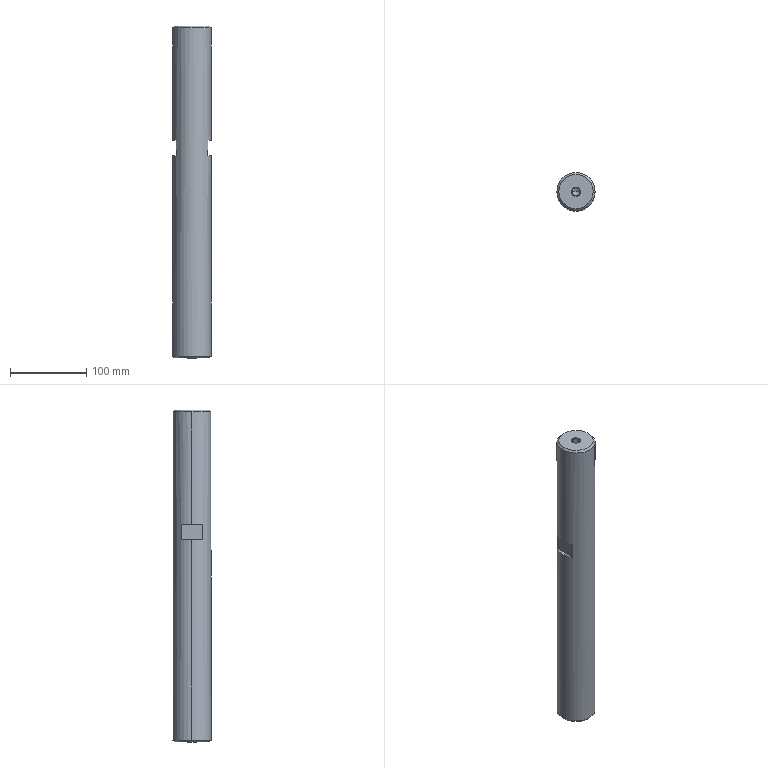Part | STEP file | RAD36-D50-L435-SC150-M12-N12-Yiheda | 1 solid | 26 faces | box 50 x 50 x 435 mm | volume 845554 mm3 | cone 12 | plane 8 | cylinder 6 | commonest cylinder face diameters 10.106 x4 50 x2
STEP:
#1=CARTESIAN_POINT('',(-25.,0.,-2.5));
#2=VERTEX_POINT('',#1);
#3=CARTESIAN_POINT('',(25.,0.,-2.5));
#4=VERTEX_POINT('',#3);
#5=CARTESIAN_POINT('',(0.,0.,-2.5));
#6=DIRECTION('',(0.,0.,-1.));
#7=DIRECTION('',(-1.,0.,0.));
#8=AXIS2_PLACEMENT_3D('',#5,#6,#7);
#9=CIRCLE('',#8,25.);
#10=EDGE_CURVE('',#2,#4,#9,.T.);
#11=ORIENTED_EDGE('',*,*,#10,.T.);
#12=CARTESIAN_POINT('',(25.,0.,-150.));
#13=VERTEX_POINT('',#12);
#14=CARTESIAN_POINT('',(25.,0.,-600.));
#15=DIRECTION('',(0.,0.,-1.));
#16=VECTOR('',#15,1000.);
#17=LINE('',#14,#16);
#18=EDGE_CURVE('',#4,#13,#17,.T.);
#19=ORIENTED_EDGE('',*,*,#18,.T.);
#20=CARTESIAN_POINT('',(20.5,14.309,-150.));
#21=VERTEX_POINT('',#20);
#22=CARTESIAN_POINT('',(0.,0.,-150.));
#23=DIRECTION('',(0.,0.,1.));
#24=DIRECTION('',(-1.,0.,0.));
#25=AXIS2_PLACEMENT_3D('',#22,#23,#24);
#26=CIRCLE('',#25,25.);
#27=EDGE_CURVE('',#13,#21,#26,.T.);
#28=ORIENTED_EDGE('',*,*,#27,.T.);
#29=CARTESIAN_POINT('',(20.5,14.309,-170.));
#30=VERTEX_POINT('',#29);
#31=CARTESIAN_POINT('',(20.5,14.309,-600.));
#32=DIRECTION('',(0.,0.,-1.));
#33=VECTOR('',#32,1000.);
#34=LINE('',#31,#33);
#35=EDGE_CURVE('',#21,#30,#34,.T.);
#36=ORIENTED_EDGE('',*,*,#35,.T.);
#37=CARTESIAN_POINT('',(25.,0.,-170.));
#38=VERTEX_POINT('',#37);
#39=CARTESIAN_POINT('',(0.,0.,-170.));
#40=DIRECTION('',(0.,0.,-1.));
#41=DIRECTION('',(-1.,0.,0.));
#42=AXIS2_PLACEMENT_3D('',#39,#40,#41);
#43=CIRCLE('',#42,25.);
#44=EDGE_CURVE('',#30,#38,#43,.T.);
#45=ORIENTED_EDGE('',*,*,#44,.T.);
#46=CARTESIAN_POINT('',(25.,0.,-432.5));
#47=VERTEX_POINT('',#46);
#48=CARTESIAN_POINT('',(25.,0.,-600.));
#49=DIRECTION('',(0.,0.,-1.));
#50=VECTOR('',#49,1000.);
#51=LINE('',#48,#50);
#52=EDGE_CURVE('',#38,#47,#51,.T.);
#53=ORIENTED_EDGE('',*,*,#52,.T.);
#54=CARTESIAN_POINT('',(0.,25.,-432.5));
#55=VERTEX_POINT('',#54);
#56=CARTESIAN_POINT('',(0.,0.,-432.5));
#57=DIRECTION('',(0.,0.,1.));
#58=DIRECTION('',(-1.,0.,0.));
#59=AXIS2_PLACEMENT_3D('',#56,#57,#58);
#60=CIRCLE('',#59,25.);
#61=EDGE_CURVE('',#47,#55,#60,.T.);
#62=ORIENTED_EDGE('',*,*,#61,.T.);
#63=CARTESIAN_POINT('',(-25.,0.,-432.5));
#64=VERTEX_POINT('',#63);
#65=CARTESIAN_POINT('',(0.,0.,-432.5));
#66=DIRECTION('',(0.,0.,1.));
#67=DIRECTION('',(-1.,0.,0.));
#68=AXIS2_PLACEMENT_3D('',#65,#66,#67);
#69=CIRCLE('',#68,25.);
#70=EDGE_CURVE('',#55,#64,#69,.T.);
#71=ORIENTED_EDGE('',*,*,#70,.T.);
#72=CARTESIAN_POINT('',(-25.,0.,-170.));
#73=VERTEX_POINT('',#72);
#74=CARTESIAN_POINT('',(-25.,0.,-600.));
#75=DIRECTION('',(0.,0.,-1.));
#76=VECTOR('',#75,1000.);
#77=LINE('',#74,#76);
#78=EDGE_CURVE('',#73,#64,#77,.T.);
#79=ORIENTED_EDGE('',*,*,#78,.F.);
#80=CARTESIAN_POINT('',(-20.5,14.309,-170.));
#81=VERTEX_POINT('',#80);
#82=CARTESIAN_POINT('',(0.,0.,-170.));
#83=DIRECTION('',(0.,0.,-1.));
#84=DIRECTION('',(-1.,0.,0.));
#85=AXIS2_PLACEMENT_3D('',#82,#83,#84);
#86=CIRCLE('',#85,25.);
#87=EDGE_CURVE('',#73,#81,#86,.T.);
#88=ORIENTED_EDGE('',*,*,#87,.T.);
#89=CARTESIAN_POINT('',(-20.5,14.309,-150.));
#90=VERTEX_POINT('',#89);
#91=CARTESIAN_POINT('',(-20.5,14.309,-600.));
#92=DIRECTION('',(0.,0.,1.));
#93=VECTOR('',#92,1000.);
#94=LINE('',#91,#93);
#95=EDGE_CURVE('',#81,#90,#94,.T.);
#96=ORIENTED_EDGE('',*,*,#95,.T.);
#97=CARTESIAN_POINT('',(-25.,0.,-150.));
#98=VERTEX_POINT('',#97);
#99=CARTESIAN_POINT('',(0.,0.,-150.));
#100=DIRECTION('',(0.,0.,1.));
#101=DIRECTION('',(-1.,0.,0.));
#102=AXIS2_PLACEMENT_3D('',#99,#100,#101);
#103=CIRCLE('',#102,25.);
#104=EDGE_CURVE('',#90,#98,#103,.T.);
#105=ORIENTED_EDGE('',*,*,#104,.T.);
#106=CARTESIAN_POINT('',(-25.,0.,-600.));
#107=DIRECTION('',(0.,0.,-1.));
#108=VECTOR('',#107,1000.);
#109=LINE('',#106,#108);
#110=EDGE_CURVE('',#2,#98,#109,.T.);
#111=ORIENTED_EDGE('',*,*,#110,.F.);
#112=EDGE_LOOP('',(#11,#19,#28,#36,#45,#53,#62,#71,#79,#88,#96,#105,#111));
#113=FACE_OUTER_BOUND('',#112,.T.);
#114=CARTESIAN_POINT('',(0.,0.,-600.));
#115=DIRECTION('',(0.,0.,-1.));
#116=DIRECTION('',(-1.,0.,0.));
#117=AXIS2_PLACEMENT_3D('',#114,#115,#116);
#118=CYLINDRICAL_SURFACE('',#117,25.);
#119=ADVANCED_FACE('',(#113),#118,.T.);
#120=CARTESIAN_POINT('',(-22.5,0.,0.));
#121=VERTEX_POINT('',#120);
#122=CARTESIAN_POINT('',(22.5,0.,0.));
#123=VERTEX_POINT('',#122);
#124=CARTESIAN_POINT('',(0.,0.,0.));
#125=DIRECTION('',(0.,0.,-1.));
#126=DIRECTION('',(-1.,0.,0.));
#127=AXIS2_PLACEMENT_3D('',#124,#125,#126);
#128=CIRCLE('',#127,22.5);
#129=EDGE_CURVE('',#121,#123,#128,.T.);
#130=ORIENTED_EDGE('',*,*,#129,.T.);
#131=CARTESIAN_POINT('',(25.,0.,-2.5));
#132=DIRECTION('',(0.7071,0.,-0.7071));
#133=VECTOR('',#132,1000.);
#134=LINE('',#131,#133);
#135=EDGE_CURVE('',#123,#4,#134,.T.);
#136=ORIENTED_EDGE('',*,*,#135,.T.);
#137=ORIENTED_EDGE('',*,*,#10,.F.);
#138=CARTESIAN_POINT('',(-25.,0.,-2.5));
#139=DIRECTION('',(-0.7071,0.,-0.7071));
#140=VECTOR('',#139,1000.);
#141=LINE('',#138,#140);
#142=EDGE_CURVE('',#121,#2,#141,.T.);
#143=ORIENTED_EDGE('',*,*,#142,.F.);
#144=EDGE_LOOP('',(#130,#136,#137,#143));
#145=FACE_OUTER_BOUND('',#144,.T.);
#146=CARTESIAN_POINT('',(0.,0.,-2.5));
#147=DIRECTION('',(0.,0.,-1.));
#148=DIRECTION('',(-1.,0.,0.));
#149=AXIS2_PLACEMENT_3D('',#146,#147,#148);
#150=CONICAL_SURFACE('',#149,25.,0.7854);
#151=ADVANCED_FACE('',(#145),#150,.T.);
#152=CARTESIAN_POINT('',(0.,-22.5,-435.));
#153=VERTEX_POINT('',#152);
#154=CARTESIAN_POINT('',(0.,22.5,-435.));
#155=VERTEX_POINT('',#154);
#156=CARTESIAN_POINT('',(0.,0.,-435.));
#157=DIRECTION('',(0.,0.,1.));
#158=DIRECTION('',(0.,-1.,0.));
#159=AXIS2_PLACEMENT_3D('',#156,#157,#158);
#160=CIRCLE('',#159,22.5);
#161=EDGE_CURVE('',#153,#155,#160,.T.);
#162=ORIENTED_EDGE('',*,*,#161,.T.);
#163=CARTESIAN_POINT('',(0.,25.,-432.5));
#164=DIRECTION('',(0.,0.7071,0.7071));
#165=VECTOR('',#164,1000.);
#166=LINE('',#163,#165);
#167=EDGE_CURVE('',#155,#55,#166,.T.);
#168=ORIENTED_EDGE('',*,*,#167,.T.);
#169=ORIENTED_EDGE('',*,*,#61,.F.);
#170=CARTESIAN_POINT('',(0.,-25.,-432.5));
#171=VERTEX_POINT('',#170);
#172=CARTESIAN_POINT('',(0.,0.,-432.5));
#173=DIRECTION('',(0.,0.,1.));
#174=DIRECTION('',(-1.,0.,0.));
#175=AXIS2_PLACEMENT_3D('',#172,#173,#174);
#176=CIRCLE('',#175,25.);
#177=EDGE_CURVE('',#171,#47,#176,.T.);
#178=ORIENTED_EDGE('',*,*,#177,.F.);
#179=CARTESIAN_POINT('',(0.,-25.,-432.5));
#180=DIRECTION('',(0.,-0.7071,0.7071));
#181=VECTOR('',#180,1000.);
#182=LINE('',#179,#181);
#183=EDGE_CURVE('',#153,#171,#182,.T.);
#184=ORIENTED_EDGE('',*,*,#183,.F.);
#185=EDGE_LOOP('',(#162,#168,#169,#178,#184));
#186=FACE_OUTER_BOUND('',#185,.T.);
#187=CARTESIAN_POINT('',(0.,0.,-432.5));
#188=DIRECTION('',(0.,0.,1.));
#189=DIRECTION('',(0.,-1.,0.));
#190=AXIS2_PLACEMENT_3D('',#187,#188,#189);
#191=CONICAL_SURFACE('',#190,25.,0.7854);
#192=ADVANCED_FACE('',(#186),#191,.T.);
#193=CARTESIAN_POINT('',(0.,5.053,-0.947));
#194=VERTEX_POINT('',#193);
#195=CARTESIAN_POINT('',(0.,-5.053,-0.947));
#196=VERTEX_POINT('',#195);
#197=CARTESIAN_POINT('',(0.,0.,-0.947));
#198=DIRECTION('',(0.,0.,1.));
#199=DIRECTION('',(0.,-1.,0.));
#200=AXIS2_PLACEMENT_3D('',#197,#198,#199);
#201=CIRCLE('',#200,5.053);
#202=EDGE_CURVE('',#194,#196,#201,.T.);
#203=ORIENTED_EDGE('',*,*,#202,.F.);
#204=CARTESIAN_POINT('',(0.,6.,0.));
#205=VERTEX_POINT('',#204);
#206=CARTESIAN_POINT('',(0.,6.,0.));
#207=DIRECTION('',(0.,0.7071,0.7071));
#208=VECTOR('',#207,1000.);
#209=LINE('',#206,#208);
#210=EDGE_CURVE('',#194,#205,#209,.T.);
#211=ORIENTED_EDGE('',*,*,#210,.T.);
#212=CARTESIAN_POINT('',(0.,-6.,0.));
#213=VERTEX_POINT('',#212);
#214=CARTESIAN_POINT('',(0.,0.,0.));
#215=DIRECTION('',(0.,0.,1.));
#216=DIRECTION('',(0.,-1.,0.));
#217=AXIS2_PLACEMENT_3D('',#214,#215,#216);
#218=CIRCLE('',#217,6.);
#219=EDGE_CURVE('',#205,#213,#218,.T.);
#220=ORIENTED_EDGE('',*,*,#219,.T.);
#221=CARTESIAN_POINT('',(0.,-6.,0.));
#222=DIRECTION('',(0.,-0.7071,0.7071));
#223=VECTOR('',#222,1000.);
#224=LINE('',#221,#223);
#225=EDGE_CURVE('',#196,#213,#224,.T.);
#226=ORIENTED_EDGE('',*,*,#225,.F.);
#227=EDGE_LOOP('',(#203,#211,#220,#226));
#228=FACE_OUTER_BOUND('',#227,.T.);
#229=CARTESIAN_POINT('',(0.,0.,0.));
#230=DIRECTION('',(0.,0.,1.));
#231=DIRECTION('',(0.,-1.,0.));
#232=AXIS2_PLACEMENT_3D('',#229,#230,#231);
#233=CONICAL_SURFACE('',#232,6.,0.7854);
#234=ADVANCED_FACE('',(#228),#233,.F.);
#235=CARTESIAN_POINT('',(5.053,0.,-434.053));
#236=VERTEX_POINT('',#235);
#237=CARTESIAN_POINT('',(0.,-5.053,-434.053));
#238=VERTEX_POINT('',#237);
#239=CARTESIAN_POINT('',(0.,0.,-434.053));
#240=DIRECTION('',(0.,0.,-1.));
#241=DIRECTION('',(0.,1.,0.));
#242=AXIS2_PLACEMENT_3D('',#239,#240,#241);
#243=CIRCLE('',#242,5.053);
#244=EDGE_CURVE('',#236,#238,#243,.T.);
#245=ORIENTED_EDGE('',*,*,#244,.F.);
#246=CARTESIAN_POINT('',(6.,0.,-435.));
#247=VERTEX_POINT('',#246);
#248=CARTESIAN_POINT('',(6.,0.,-435.));
#249=DIRECTION('',(0.7071,0.,-0.7071));
#250=VECTOR('',#249,1000.);
#251=LINE('',#248,#250);
#252=EDGE_CURVE('',#236,#247,#251,.T.);
#253=ORIENTED_EDGE('',*,*,#252,.T.);
#254=CARTESIAN_POINT('',(-6.,0.,-435.));
#255=VERTEX_POINT('',#254);
#256=CARTESIAN_POINT('',(0.,0.,-435.));
#257=DIRECTION('',(0.,0.,-1.));
#258=DIRECTION('',(-1.,0.,0.));
#259=AXIS2_PLACEMENT_3D('',#256,#257,#258);
#260=CIRCLE('',#259,6.);
#261=EDGE_CURVE('',#247,#255,#260,.T.);
#262=ORIENTED_EDGE('',*,*,#261,.T.);
#263=CARTESIAN_POINT('',(-5.053,0.,-434.053));
#264=VERTEX_POINT('',#263);
#265=CARTESIAN_POINT('',(-6.,0.,-435.));
#266=DIRECTION('',(-0.7071,0.,-0.7071));
#267=VECTOR('',#266,1000.);
#268=LINE('',#265,#267);
#269=EDGE_CURVE('',#264,#255,#268,.T.);
#270=ORIENTED_EDGE('',*,*,#269,.F.);
#271=CARTESIAN_POINT('',(0.,0.,-434.053));
#272=DIRECTION('',(0.,0.,-1.));
#273=DIRECTION('',(0.,1.,0.));
#274=AXIS2_PLACEMENT_3D('',#271,#272,#273);
#275=CIRCLE('',#274,5.053);
#276=EDGE_CURVE('',#238,#264,#275,.T.);
#277=ORIENTED_EDGE('',*,*,#276,.F.);
#278=EDGE_LOOP('',(#245,#253,#262,#270,#277));
#279=FACE_OUTER_BOUND('',#278,.T.);
#280=CARTESIAN_POINT('',(0.,0.,-435.));
#281=DIRECTION('',(0.,0.,-1.));
#282=DIRECTION('',(-1.,0.,0.));
#283=AXIS2_PLACEMENT_3D('',#280,#281,#282);
#284=CONICAL_SURFACE('',#283,6.,0.7854);
#285=ADVANCED_FACE('',(#279),#284,.F.);
#286=ORIENTED_EDGE('',*,*,#202,.T.);
#287=CARTESIAN_POINT('',(0.,-5.053,-24.5));
#288=VERTEX_POINT('',#287);
#289=CARTESIAN_POINT('',(0.,-5.053,-27.417));
#290=DIRECTION('',(0.,0.,-1.));
#291=VECTOR('',#290,1000.);
#292=LINE('',#289,#291);
#293=EDGE_CURVE('',#196,#288,#292,.T.);
#294=ORIENTED_EDGE('',*,*,#293,.T.);
#295=CARTESIAN_POINT('',(-5.053,0.,-24.5));
#296=VERTEX_POINT('',#295);
#297=CARTESIAN_POINT('',(0.,0.,-24.5));
#298=DIRECTION('',(0.,0.,1.));
#299=DIRECTION('',(0.,1.,0.));
#300=AXIS2_PLACEMENT_3D('',#297,#298,#299);
#301=CIRCLE('',#300,5.053);
#302=EDGE_CURVE('',#296,#288,#301,.T.);
#303=ORIENTED_EDGE('',*,*,#302,.F.);
#304=CARTESIAN_POINT('',(0.,5.053,-24.5));
#305=VERTEX_POINT('',#304);
#306=CARTESIAN_POINT('',(0.,0.,-24.5));
#307=DIRECTION('',(0.,0.,1.));
#308=DIRECTION('',(0.,1.,0.));
#309=AXIS2_PLACEMENT_3D('',#306,#307,#308);
#310=CIRCLE('',#309,5.053);
#311=EDGE_CURVE('',#305,#296,#310,.T.);
#312=ORIENTED_EDGE('',*,*,#311,.F.);
#313=CARTESIAN_POINT('',(0.,5.053,-27.417));
#314=DIRECTION('',(0.,0.,-1.));
#315=VECTOR('',#314,1000.);
#316=LINE('',#313,#315);
#317=EDGE_CURVE('',#194,#305,#316,.T.);
#318=ORIENTED_EDGE('',*,*,#317,.F.);
#319=EDGE_LOOP('',(#286,#294,#303,#312,#318));
#320=FACE_OUTER_BOUND('',#319,.T.);
#321=CARTESIAN_POINT('',(0.,0.,-27.417));
#322=DIRECTION('',(0.,0.,-1.));
#323=DIRECTION('',(0.,1.,0.));
#324=AXIS2_PLACEMENT_3D('',#321,#322,#323);
#325=CYLINDRICAL_SURFACE('',#324,5.053);
#326=ADVANCED_FACE('',(#320),#325,.F.);
#327=CARTESIAN_POINT('',(0.,-5.053,-410.5));
#328=VERTEX_POINT('',#327);
#329=CARTESIAN_POINT('',(-5.053,0.,-410.5));
#330=VERTEX_POINT('',#329);
#331=CARTESIAN_POINT('',(0.,0.,-410.5));
#332=DIRECTION('',(0.,0.,-1.));
#333=DIRECTION('',(0.,1.,0.));
#334=AXIS2_PLACEMENT_3D('',#331,#332,#333);
#335=CIRCLE('',#334,5.053);
#336=EDGE_CURVE('',#328,#330,#335,.T.);
#337=ORIENTED_EDGE('',*,*,#336,.F.);
#338=CARTESIAN_POINT('',(0.,-5.053,-435.));
#339=DIRECTION('',(0.,0.,-1.));
#340=VECTOR('',#339,1000.);
#341=LINE('',#338,#340);
#342=EDGE_CURVE('',#328,#238,#341,.T.);
#343=ORIENTED_EDGE('',*,*,#342,.T.);
#344=ORIENTED_EDGE('',*,*,#276,.T.);
#345=CARTESIAN_POINT('',(0.,5.053,-434.053));
#346=VERTEX_POINT('',#345);
#347=CARTESIAN_POINT('',(0.,0.,-434.053));
#348=DIRECTION('',(0.,0.,-1.));
#349=DIRECTION('',(0.,1.,0.));
#350=AXIS2_PLACEMENT_3D('',#347,#348,#349);
#351=CIRCLE('',#350,5.053);
#352=EDGE_CURVE('',#264,#346,#351,.T.);
#353=ORIENTED_EDGE('',*,*,#352,.T.);
#354=CARTESIAN_POINT('',(0.,5.053,-410.5));
#355=VERTEX_POINT('',#354);
#356=CARTESIAN_POINT('',(0.,5.053,-435.));
#357=DIRECTION('',(0.,0.,-1.));
#358=VECTOR('',#357,1000.);
#359=LINE('',#356,#358);
#360=EDGE_CURVE('',#355,#346,#359,.T.);
#361=ORIENTED_EDGE('',*,*,#360,.F.);
#362=CARTESIAN_POINT('',(0.,0.,-410.5));
#363=DIRECTION('',(0.,0.,-1.));
#364=DIRECTION('',(0.,1.,0.));
#365=AXIS2_PLACEMENT_3D('',#362,#363,#364);
#366=CIRCLE('',#365,5.053);
#367=EDGE_CURVE('',#330,#355,#366,.T.);
#368=ORIENTED_EDGE('',*,*,#367,.F.);
#369=EDGE_LOOP('',(#337,#343,#344,#353,#361,#368));
#370=FACE_OUTER_BOUND('',#369,.T.);
#371=CARTESIAN_POINT('',(0.,0.,-435.));
#372=DIRECTION('',(0.,0.,-1.));
#373=DIRECTION('',(0.,1.,0.));
#374=AXIS2_PLACEMENT_3D('',#371,#372,#373);
#375=CYLINDRICAL_SURFACE('',#374,5.053);
#376=ADVANCED_FACE('',(#370),#375,.F.);
#377=CARTESIAN_POINT('',(0.,0.,-27.417));
#378=VERTEX_POINT('',#377);
#379=CARTESIAN_POINT('',(5.053,0.,-24.5));
#380=VERTEX_POINT('',#379);
#381=CARTESIAN_POINT('',(5.053,0.,-24.5));
#382=DIRECTION('',(0.866,0.,0.5));
#383=VECTOR('',#382,1000.);
#384=LINE('',#381,#383);
#385=EDGE_CURVE('',#378,#380,#384,.T.);
#386=ORIENTED_EDGE('',*,*,#385,.F.);
#387=CARTESIAN_POINT('',(-5.053,0.,-24.5));
#388=DIRECTION('',(-0.866,0.,0.5));
#389=VECTOR('',#388,1000.);
#390=LINE('',#387,#389);
#391=EDGE_CURVE('',#378,#296,#390,.T.);
#392=ORIENTED_EDGE('',*,*,#391,.T.);
#393=ORIENTED_EDGE('',*,*,#302,.T.);
#394=CARTESIAN_POINT('',(0.,0.,-24.5));
#395=DIRECTION('',(0.,0.,1.));
#396=DIRECTION('',(0.,1.,0.));
#397=AXIS2_PLACEMENT_3D('',#394,#395,#396);
#398=CIRCLE('',#397,5.053);
#399=EDGE_CURVE('',#288,#380,#398,.T.);
#400=ORIENTED_EDGE('',*,*,#399,.T.);
#401=EDGE_LOOP('',(#386,#392,#393,#400));
#402=FACE_OUTER_BOUND('',#401,.T.);
#403=CARTESIAN_POINT('',(0.,0.,-24.5));
#404=DIRECTION('',(0.,0.,1.));
#405=DIRECTION('',(1.,0.,0.));
#406=AXIS2_PLACEMENT_3D('',#403,#404,#405);
#407=CONICAL_SURFACE('',#406,5.053,1.047);
#408=ADVANCED_FACE('',(#402),#407,.F.);
#409=CARTESIAN_POINT('',(0.,0.,-407.583));
#410=VERTEX_POINT('',#409);
#411=CARTESIAN_POINT('',(-5.053,0.,-410.5));
#412=DIRECTION('',(-0.866,0.,-0.5));
#413=VECTOR('',#412,1000.);
#414=LINE('',#411,#413);
#415=EDGE_CURVE('',#410,#330,#414,.T.);
#416=ORIENTED_EDGE('',*,*,#415,.F.);
#417=CARTESIAN_POINT('',(5.053,0.,-410.5));
#418=VERTEX_POINT('',#417);
#419=CARTESIAN_POINT('',(5.053,0.,-410.5));
#420=DIRECTION('',(0.866,0.,-0.5));
#421=VECTOR('',#420,1000.);
#422=LINE('',#419,#421);
#423=EDGE_CURVE('',#410,#418,#422,.T.);
#424=ORIENTED_EDGE('',*,*,#423,.T.);
#425=CARTESIAN_POINT('',(0.,0.,-410.5));
#426=DIRECTION('',(0.,0.,-1.));
#427=DIRECTION('',(0.,1.,0.));
#428=AXIS2_PLACEMENT_3D('',#425,#426,#427);
#429=CIRCLE('',#428,5.053);
#430=EDGE_CURVE('',#418,#328,#429,.T.);
#431=ORIENTED_EDGE('',*,*,#430,.T.);
#432=ORIENTED_EDGE('',*,*,#336,.T.);
#433=EDGE_LOOP('',(#416,#424,#431,#432));
#434=FACE_OUTER_BOUND('',#433,.T.);
#435=CARTESIAN_POINT('',(0.,0.,-410.5));
#436=DIRECTION('',(0.,0.,-1.));
#437=DIRECTION('',(-1.,0.,0.));
#438=AXIS2_PLACEMENT_3D('',#435,#436,#437);
#439=CONICAL_SURFACE('',#438,5.053,1.047);
#440=ADVANCED_FACE('',(#434),#439,.F.);
#441=ORIENTED_EDGE('',*,*,#18,.F.);
#442=CARTESIAN_POINT('',(0.,0.,-2.5));
#443=DIRECTION('',(0.,0.,-1.));
#444=DIRECTION('',(-1.,0.,0.));
#445=AXIS2_PLACEMENT_3D('',#442,#443,#444);
#446=CIRCLE('',#445,25.);
#447=EDGE_CURVE('',#4,#2,#446,.T.);
#448=ORIENTED_EDGE('',*,*,#447,.T.);
#449=ORIENTED_EDGE('',*,*,#110,.T.);
#450=CARTESIAN_POINT('',(-20.5,-14.309,-150.));
#451=VERTEX_POINT('',#450);
#452=CARTESIAN_POINT('',(0.,0.,-150.));
#453=DIRECTION('',(0.,0.,1.));
#454=DIRECTION('',(-1.,0.,0.));
#455=AXIS2_PLACEMENT_3D('',#452,#453,#454);
#456=CIRCLE('',#455,25.);
#457=EDGE_CURVE('',#98,#451,#456,.T.);
#458=ORIENTED_EDGE('',*,*,#457,.T.);
#459=CARTESIAN_POINT('',(-20.5,-14.309,-170.));
#460=VERTEX_POINT('',#459);
#461=CARTESIAN_POINT('',(-20.5,-14.309,-600.));
#462=DIRECTION('',(0.,0.,-1.));
#463=VECTOR('',#462,1000.);
#464=LINE('',#461,#463);
#465=EDGE_CURVE('',#451,#460,#464,.T.);
#466=ORIENTED_EDGE('',*,*,#465,.T.);
#467=CARTESIAN_POINT('',(0.,0.,-170.));
#468=DIRECTION('',(0.,0.,-1.));
#469=DIRECTION('',(-1.,0.,0.));
#470=AXIS2_PLACEMENT_3D('',#467,#468,#469);
#471=CIRCLE('',#470,25.);
#472=EDGE_CURVE('',#460,#73,#471,.T.);
#473=ORIENTED_EDGE('',*,*,#472,.T.);
#474=ORIENTED_EDGE('',*,*,#78,.T.);
#475=CARTESIAN_POINT('',(0.,0.,-432.5));
#476=DIRECTION('',(0.,0.,1.));
#477=DIRECTION('',(-1.,0.,0.));
#478=AXIS2_PLACEMENT_3D('',#475,#476,#477);
#479=CIRCLE('',#478,25.);
#480=EDGE_CURVE('',#64,#171,#479,.T.);
#481=ORIENTED_EDGE('',*,*,#480,.T.);
#482=ORIENTED_EDGE('',*,*,#177,.T.);
#483=ORIENTED_EDGE('',*,*,#52,.F.);
#484=CARTESIAN_POINT('',(20.5,-14.309,-170.));
#485=VERTEX_POINT('',#484);
#486=CARTESIAN_POINT('',(0.,0.,-170.));
#487=DIRECTION('',(0.,0.,-1.));
#488=DIRECTION('',(-1.,0.,0.));
#489=AXIS2_PLACEMENT_3D('',#486,#487,#488);
#490=CIRCLE('',#489,25.);
#491=EDGE_CURVE('',#38,#485,#490,.T.);
#492=ORIENTED_EDGE('',*,*,#491,.T.);
#493=CARTESIAN_POINT('',(20.5,-14.309,-150.));
#494=VERTEX_POINT('',#493);
#495=CARTESIAN_POINT('',(20.5,-14.309,-600.));
#496=DIRECTION('',(0.,0.,1.));
#497=VECTOR('',#496,1000.);
#498=LINE('',#495,#497);
#499=EDGE_CURVE('',#485,#494,#498,.T.);
#500=ORIENTED_EDGE('',*,*,#499,.T.);
#501=CARTESIAN_POINT('',(0.,0.,-150.));
#502=DIRECTION('',(0.,0.,1.));
#503=DIRECTION('',(-1.,0.,0.));
#504=AXIS2_PLACEMENT_3D('',#501,#502,#503);
#505=CIRCLE('',#504,25.);
#506=EDGE_CURVE('',#494,#13,#505,.T.);
#507=ORIENTED_EDGE('',*,*,#506,.T.);
#508=EDGE_LOOP('',(#441,#448,#449,#458,#466,#473,#474,#481,#482,#483,#492,#500,#507));
#509=FACE_OUTER_BOUND('',#508,.T.);
#510=CARTESIAN_POINT('',(0.,0.,-600.));
#511=DIRECTION('',(0.,0.,-1.));
#512=DIRECTION('',(-1.,0.,0.));
#513=AXIS2_PLACEMENT_3D('',#510,#511,#512);
#514=CYLINDRICAL_SURFACE('',#513,25.);
#515=ADVANCED_FACE('',(#509),#514,.T.);
#516=CARTESIAN_POINT('',(20.5,-14.309,-170.));
#517=DIRECTION('',(0.,1.,0.));
#518=VECTOR('',#517,1000.);
#519=LINE('',#516,#518);
#520=EDGE_CURVE('',#485,#30,#519,.T.);
#521=ORIENTED_EDGE('',*,*,#520,.T.);
#522=ORIENTED_EDGE('',*,*,#35,.F.);
#523=CARTESIAN_POINT('',(20.5,-14.309,-150.));
#524=DIRECTION('',(0.,-1.,0.));
#525=VECTOR('',#524,1000.);
#526=LINE('',#523,#525);
#527=EDGE_CURVE('',#21,#494,#526,.T.);
#528=ORIENTED_EDGE('',*,*,#527,.T.);
#529=ORIENTED_EDGE('',*,*,#499,.F.);
#530=EDGE_LOOP('',(#521,#522,#528,#529));
#531=FACE_OUTER_BOUND('',#530,.T.);
#532=CARTESIAN_POINT('',(20.5,-14.309,-170.));
#533=DIRECTION('',(1.,0.,0.));
#534=DIRECTION('',(0.,0.,-1.));
#535=AXIS2_PLACEMENT_3D('',#532,#533,#534);
#536=PLANE('',#535);
#537=ADVANCED_FACE('',(#531),#536,.T.);
#538=ORIENTED_EDGE('',*,*,#44,.F.);
#539=ORIENTED_EDGE('',*,*,#520,.F.);
#540=ORIENTED_EDGE('',*,*,#491,.F.);
#541=EDGE_LOOP('',(#538,#539,#540));
#542=FACE_OUTER_BOUND('',#541,.T.);
#543=CARTESIAN_POINT('',(0.,0.,-170.));
#544=DIRECTION('',(0.,0.,1.));
#545=DIRECTION('',(1.,0.,0.));
#546=AXIS2_PLACEMENT_3D('',#543,#544,#545);
#547=PLANE('',#546);
#548=ADVANCED_FACE('',(#542),#547,.T.);
#549=ORIENTED_EDGE('',*,*,#506,.F.);
#550=ORIENTED_EDGE('',*,*,#527,.F.);
#551=ORIENTED_EDGE('',*,*,#27,.F.);
#552=EDGE_LOOP('',(#549,#550,#551));
#553=FACE_OUTER_BOUND('',#552,.T.);
#554=CARTESIAN_POINT('',(0.,0.,-150.));
#555=DIRECTION('',(0.,0.,1.));
#556=DIRECTION('',(1.,0.,0.));
#557=AXIS2_PLACEMENT_3D('',#554,#555,#556);
#558=PLANE('',#557);
#559=ADVANCED_FACE('',(#553),#558,.F.);
#560=CARTESIAN_POINT('',(-20.5,14.309,-170.));
#561=DIRECTION('',(0.,-1.,0.));
#562=VECTOR('',#561,1000.);
#563=LINE('',#560,#562);
#564=EDGE_CURVE('',#81,#460,#563,.T.);
#565=ORIENTED_EDGE('',*,*,#564,.T.);
#566=ORIENTED_EDGE('',*,*,#465,.F.);
#567=CARTESIAN_POINT('',(-20.5,14.309,-150.));
#568=DIRECTION('',(0.,1.,0.));
#569=VECTOR('',#568,1000.);
#570=LINE('',#567,#569);
#571=EDGE_CURVE('',#451,#90,#570,.T.);
#572=ORIENTED_EDGE('',*,*,#571,.T.);
#573=ORIENTED_EDGE('',*,*,#95,.F.);
#574=EDGE_LOOP('',(#565,#566,#572,#573));
#575=FACE_OUTER_BOUND('',#574,.T.);
#576=CARTESIAN_POINT('',(-20.5,14.309,-170.));
#577=DIRECTION('',(-1.,0.,0.));
#578=DIRECTION('',(0.,0.,1.));
#579=AXIS2_PLACEMENT_3D('',#576,#577,#578);
#580=PLANE('',#579);
#581=ADVANCED_FACE('',(#575),#580,.T.);
#582=ORIENTED_EDGE('',*,*,#104,.F.);
#583=ORIENTED_EDGE('',*,*,#571,.F.);
#584=ORIENTED_EDGE('',*,*,#457,.F.);
#585=EDGE_LOOP('',(#582,#583,#584));
#586=FACE_OUTER_BOUND('',#585,.T.);
#587=CARTESIAN_POINT('',(0.,0.,-150.));
#588=DIRECTION('',(0.,0.,1.));
#589=DIRECTION('',(1.,0.,0.));
#590=AXIS2_PLACEMENT_3D('',#587,#588,#589);
#591=PLANE('',#590);
#592=ADVANCED_FACE('',(#586),#591,.F.);
#593=ORIENTED_EDGE('',*,*,#472,.F.);
#594=ORIENTED_EDGE('',*,*,#564,.F.);
#595=ORIENTED_EDGE('',*,*,#87,.F.);
#596=EDGE_LOOP('',(#593,#594,#595));
#597=FACE_OUTER_BOUND('',#596,.T.);
#598=CARTESIAN_POINT('',(0.,0.,-170.));
#599=DIRECTION('',(0.,0.,1.));
#600=DIRECTION('',(1.,0.,0.));
#601=AXIS2_PLACEMENT_3D('',#598,#599,#600);
#602=PLANE('',#601);
#603=ADVANCED_FACE('',(#597),#602,.T.);
#604=ORIENTED_EDGE('',*,*,#135,.F.);
#605=CARTESIAN_POINT('',(0.,0.,0.));
#606=DIRECTION('',(0.,0.,-1.));
#607=DIRECTION('',(-1.,0.,0.));
#608=AXIS2_PLACEMENT_3D('',#605,#606,#607);
#609=CIRCLE('',#608,22.5);
#610=EDGE_CURVE('',#123,#121,#609,.T.);
#611=ORIENTED_EDGE('',*,*,#610,.T.);
#612=ORIENTED_EDGE('',*,*,#142,.T.);
#613=ORIENTED_EDGE('',*,*,#447,.F.);
#614=EDGE_LOOP('',(#604,#611,#612,#613));
#615=FACE_OUTER_BOUND('',#614,.T.);
#616=CARTESIAN_POINT('',(0.,0.,-2.5));
#617=DIRECTION('',(0.,0.,-1.));
#618=DIRECTION('',(-1.,0.,0.));
#619=AXIS2_PLACEMENT_3D('',#616,#617,#618);
#620=CONICAL_SURFACE('',#619,25.,0.7854);
#621=ADVANCED_FACE('',(#615),#620,.T.);
#622=ORIENTED_EDGE('',*,*,#167,.F.);
#623=CARTESIAN_POINT('',(0.,0.,-435.));
#624=DIRECTION('',(0.,0.,1.));
#625=DIRECTION('',(0.,-1.,0.));
#626=AXIS2_PLACEMENT_3D('',#623,#624,#625);
#627=CIRCLE('',#626,22.5);
#628=EDGE_CURVE('',#155,#153,#627,.T.);
#629=ORIENTED_EDGE('',*,*,#628,.T.);
#630=ORIENTED_EDGE('',*,*,#183,.T.);
#631=ORIENTED_EDGE('',*,*,#480,.F.);
#632=ORIENTED_EDGE('',*,*,#70,.F.);
#633=EDGE_LOOP('',(#622,#629,#630,#631,#632));
#634=FACE_OUTER_BOUND('',#633,.T.);
#635=CARTESIAN_POINT('',(0.,0.,-432.5));
#636=DIRECTION('',(0.,0.,1.));
#637=DIRECTION('',(0.,-1.,0.));
#638=AXIS2_PLACEMENT_3D('',#635,#636,#637);
#639=CONICAL_SURFACE('',#638,25.,0.7854);
#640=ADVANCED_FACE('',(#634),#639,.T.);
#641=CARTESIAN_POINT('',(0.,0.,0.));
#642=DIRECTION('',(0.,0.,1.));
#643=DIRECTION('',(0.,-1.,0.));
#644=AXIS2_PLACEMENT_3D('',#641,#642,#643);
#645=CIRCLE('',#644,6.);
#646=EDGE_CURVE('',#213,#205,#645,.T.);
#647=ORIENTED_EDGE('',*,*,#646,.F.);
#648=ORIENTED_EDGE('',*,*,#219,.F.);
#649=EDGE_LOOP('',(#647,#648));
#650=FACE_BOUND('',#649,.T.);
#651=ORIENTED_EDGE('',*,*,#129,.F.);
#652=ORIENTED_EDGE('',*,*,#610,.F.);
#653=EDGE_LOOP('',(#651,#652));
#654=FACE_OUTER_BOUND('',#653,.T.);
#655=CARTESIAN_POINT('',(0.,0.,0.));
#656=DIRECTION('',(0.,0.,-1.));
#657=DIRECTION('',(-1.,0.,0.));
#658=AXIS2_PLACEMENT_3D('',#655,#656,#657);
#659=PLANE('',#658);
#660=ADVANCED_FACE('',(#650,#654),#659,.F.);
#661=ORIENTED_EDGE('',*,*,#161,.F.);
#662=ORIENTED_EDGE('',*,*,#628,.F.);
#663=EDGE_LOOP('',(#661,#662));
#664=FACE_OUTER_BOUND('',#663,.T.);
#665=CARTESIAN_POINT('',(0.,0.,-435.));
#666=DIRECTION('',(0.,0.,-1.));
#667=DIRECTION('',(-1.,0.,0.));
#668=AXIS2_PLACEMENT_3D('',#665,#666,#667);
#669=CIRCLE('',#668,6.);
#670=EDGE_CURVE('',#255,#247,#669,.T.);
#671=ORIENTED_EDGE('',*,*,#670,.F.);
#672=ORIENTED_EDGE('',*,*,#261,.F.);
#673=EDGE_LOOP('',(#671,#672));
#674=FACE_BOUND('',#673,.T.);
#675=CARTESIAN_POINT('',(0.,22.5,-435.));
#676=DIRECTION('',(0.,0.,1.));
#677=DIRECTION('',(1.,0.,0.));
#678=AXIS2_PLACEMENT_3D('',#675,#676,#677);
#679=PLANE('',#678);
#680=ADVANCED_FACE('',(#664,#674),#679,.F.);
#681=ORIENTED_EDGE('',*,*,#210,.F.);
#682=CARTESIAN_POINT('',(0.,0.,-0.947));
#683=DIRECTION('',(0.,0.,1.));
#684=DIRECTION('',(0.,-1.,0.));
#685=AXIS2_PLACEMENT_3D('',#682,#683,#684);
#686=CIRCLE('',#685,5.053);
#687=EDGE_CURVE('',#196,#194,#686,.T.);
#688=ORIENTED_EDGE('',*,*,#687,.F.);
#689=ORIENTED_EDGE('',*,*,#225,.T.);
#690=ORIENTED_EDGE('',*,*,#646,.T.);
#691=EDGE_LOOP('',(#681,#688,#689,#690));
#692=FACE_OUTER_BOUND('',#691,.T.);
#693=CARTESIAN_POINT('',(0.,0.,0.));
#694=DIRECTION('',(0.,0.,1.));
#695=DIRECTION('',(0.,-1.,0.));
#696=AXIS2_PLACEMENT_3D('',#693,#694,#695);
#697=CONICAL_SURFACE('',#696,6.,0.7854);
#698=ADVANCED_FACE('',(#692),#697,.F.);
#699=ORIENTED_EDGE('',*,*,#252,.F.);
#700=CARTESIAN_POINT('',(0.,0.,-434.053));
#701=DIRECTION('',(0.,0.,-1.));
#702=DIRECTION('',(0.,1.,0.));
#703=AXIS2_PLACEMENT_3D('',#700,#701,#702);
#704=CIRCLE('',#703,5.053);
#705=EDGE_CURVE('',#346,#236,#704,.T.);
#706=ORIENTED_EDGE('',*,*,#705,.F.);
#707=ORIENTED_EDGE('',*,*,#352,.F.);
#708=ORIENTED_EDGE('',*,*,#269,.T.);
#709=ORIENTED_EDGE('',*,*,#670,.T.);
#710=EDGE_LOOP('',(#699,#706,#707,#708,#709));
#711=FACE_OUTER_BOUND('',#710,.T.);
#712=CARTESIAN_POINT('',(0.,0.,-435.));
#713=DIRECTION('',(0.,0.,-1.));
#714=DIRECTION('',(-1.,0.,0.));
#715=AXIS2_PLACEMENT_3D('',#712,#713,#714);
#716=CONICAL_SURFACE('',#715,6.,0.7854);
#717=ADVANCED_FACE('',(#711),#716,.F.);
#718=ORIENTED_EDGE('',*,*,#293,.F.);
#719=ORIENTED_EDGE('',*,*,#687,.T.);
#720=ORIENTED_EDGE('',*,*,#317,.T.);
#721=CARTESIAN_POINT('',(0.,0.,-24.5));
#722=DIRECTION('',(0.,0.,1.));
#723=DIRECTION('',(0.,1.,0.));
#724=AXIS2_PLACEMENT_3D('',#721,#722,#723);
#725=CIRCLE('',#724,5.053);
#726=EDGE_CURVE('',#380,#305,#725,.T.);
#727=ORIENTED_EDGE('',*,*,#726,.F.);
#728=ORIENTED_EDGE('',*,*,#399,.F.);
#729=EDGE_LOOP('',(#718,#719,#720,#727,#728));
#730=FACE_OUTER_BOUND('',#729,.T.);
#731=CARTESIAN_POINT('',(0.,0.,-27.417));
#732=DIRECTION('',(0.,0.,-1.));
#733=DIRECTION('',(0.,1.,0.));
#734=AXIS2_PLACEMENT_3D('',#731,#732,#733);
#735=CYLINDRICAL_SURFACE('',#734,5.053);
#736=ADVANCED_FACE('',(#730),#735,.F.);
#737=ORIENTED_EDGE('',*,*,#342,.F.);
#738=ORIENTED_EDGE('',*,*,#430,.F.);
#739=CARTESIAN_POINT('',(0.,0.,-410.5));
#740=DIRECTION('',(0.,0.,-1.));
#741=DIRECTION('',(0.,1.,0.));
#742=AXIS2_PLACEMENT_3D('',#739,#740,#741);
#743=CIRCLE('',#742,5.053);
#744=EDGE_CURVE('',#355,#418,#743,.T.);
#745=ORIENTED_EDGE('',*,*,#744,.F.);
#746=ORIENTED_EDGE('',*,*,#360,.T.);
#747=ORIENTED_EDGE('',*,*,#705,.T.);
#748=ORIENTED_EDGE('',*,*,#244,.T.);
#749=EDGE_LOOP('',(#737,#738,#745,#746,#747,#748));
#750=FACE_OUTER_BOUND('',#749,.T.);
#751=CARTESIAN_POINT('',(0.,0.,-435.));
#752=DIRECTION('',(0.,0.,-1.));
#753=DIRECTION('',(0.,1.,0.));
#754=AXIS2_PLACEMENT_3D('',#751,#752,#753);
#755=CYLINDRICAL_SURFACE('',#754,5.053);
#756=ADVANCED_FACE('',(#750),#755,.F.);
#757=ORIENTED_EDGE('',*,*,#391,.F.);
#758=ORIENTED_EDGE('',*,*,#385,.T.);
#759=ORIENTED_EDGE('',*,*,#726,.T.);
#760=ORIENTED_EDGE('',*,*,#311,.T.);
#761=EDGE_LOOP('',(#757,#758,#759,#760));
#762=FACE_OUTER_BOUND('',#761,.T.);
#763=CARTESIAN_POINT('',(0.,0.,-24.5));
#764=DIRECTION('',(0.,0.,1.));
#765=DIRECTION('',(1.,0.,0.));
#766=AXIS2_PLACEMENT_3D('',#763,#764,#765);
#767=CONICAL_SURFACE('',#766,5.053,1.047);
#768=ADVANCED_FACE('',(#762),#767,.F.);
#769=ORIENTED_EDGE('',*,*,#423,.F.);
#770=ORIENTED_EDGE('',*,*,#415,.T.);
#771=ORIENTED_EDGE('',*,*,#367,.T.);
#772=ORIENTED_EDGE('',*,*,#744,.T.);
#773=EDGE_LOOP('',(#769,#770,#771,#772));
#774=FACE_OUTER_BOUND('',#773,.T.);
#775=CARTESIAN_POINT('',(0.,0.,-410.5));
#776=DIRECTION('',(0.,0.,-1.));
#777=DIRECTION('',(-1.,0.,0.));
#778=AXIS2_PLACEMENT_3D('',#775,#776,#777);
#779=CONICAL_SURFACE('',#778,5.053,1.047);
#780=ADVANCED_FACE('',(#774),#779,.F.);
#781=CLOSED_SHELL('',(#119,#151,#192,#234,#285,#326,#376,#408,#440,#515,#537,#548,#559,#581,#592,#603,#621,#640,#660,#680,#698,#717,#736,#756,#768,#780));
#782=MANIFOLD_SOLID_BREP('',#781);
#783=CARTESIAN_POINT('',(0.,0.,0.));
#784=DIRECTION('',(0.,0.,1.));
#785=DIRECTION('',(1.,0.,0.));
#786=AXIS2_PLACEMENT_3D('',#783,#784,#785);
#787=(LENGTH_UNIT()NAMED_UNIT(*)SI_UNIT(.MILLI.,.METRE.));
#788=UNCERTAINTY_MEASURE_WITH_UNIT(LENGTH_MEASURE(0.00001),#787,'','');
#789=(NAMED_UNIT(*)PLANE_ANGLE_UNIT()SI_UNIT($,.RADIAN.));
#790=(NAMED_UNIT(*)SI_UNIT($,.STERADIAN.)SOLID_ANGLE_UNIT());
#791=(GEOMETRIC_REPRESENTATION_CONTEXT(3)GLOBAL_UNCERTAINTY_ASSIGNED_CONTEXT((#788))GLOBAL_UNIT_ASSIGNED_CONTEXT((#787,#789,#790))REPRESENTATION_CONTEXT('',''));
#792=ADVANCED_BREP_SHAPE_REPRESENTATION('',(#782,#786),#791);